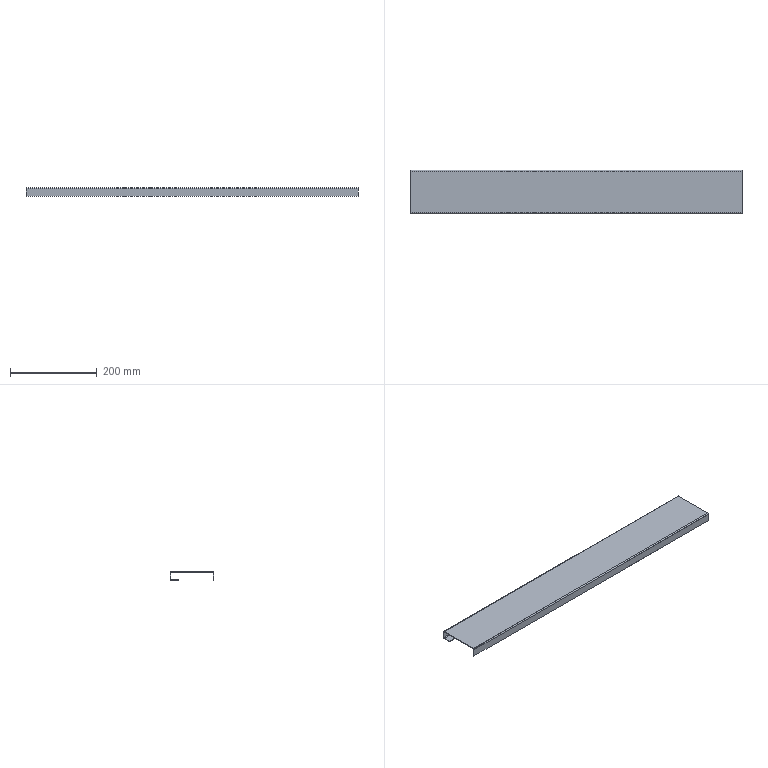Part | STEP file | E3-中转釜护栏7踢脚Plate | 1 solid | 18 faces | box 765 x 100 x 20 mm | volume 175851 mm3 | plane 12 | cylinder 6 | commonest cylinder face diameters 2 x3 5 x3
STEP:
#1=CARTESIAN_POINT('',(0.,0.,0.));
#2=DIRECTION('',(0.,0.,1.));
#3=DIRECTION('',(1.,0.,0.));
#4=AXIS2_PLACEMENT_3D('',#1,#2,#3);
#5=CARTESIAN_POINT('',(-382.5,1.5,-2.5));
#6=VERTEX_POINT('',#5);
#7=CARTESIAN_POINT('',(-382.5,1.5,-20.));
#8=VERTEX_POINT('',#7);
#9=CARTESIAN_POINT('',(-382.5,1.5,-2.5));
#10=DIRECTION('',(0.,0.,-1.));
#11=VECTOR('',#10,1.);
#12=LINE('',#9,#11);
#13=CARTESIAN_POINT('',(382.5,1.5,-2.5));
#14=DIRECTION('',(0.,-1.,0.));
#15=DIRECTION('',(0.,0.,1.));
#16=AXIS2_PLACEMENT_3D('',#13,#14,#15);
#17=PLANE('',#16);
#18=CARTESIAN_POINT('',(0.,765.));
#19=DIRECTION('',(-1.,0.));
#20=VECTOR('',#19,1.);
#21=LINE('',#18,#20);
#22=(GEOMETRIC_REPRESENTATION_CONTEXT(2)PARAMETRIC_REPRESENTATION_CONTEXT()REPRESENTATION_CONTEXT('',''));
#23=DEFINITIONAL_REPRESENTATION('',(#21),#22);
#24=PCURVE('',#17,#23);
#25=CARTESIAN_POINT('',(-382.5,2.5,-2.5));
#26=DIRECTION('',(-1.,0.,0.));
#27=DIRECTION('',(0.,0.,-1.));
#28=AXIS2_PLACEMENT_3D('',#25,#26,#27);
#29=PLANE('',#28);
#30=CARTESIAN_POINT('',(0.,1.));
#31=DIRECTION('',(1.,0.));
#32=VECTOR('',#31,1.);
#33=LINE('',#30,#32);
#34=(GEOMETRIC_REPRESENTATION_CONTEXT(2)PARAMETRIC_REPRESENTATION_CONTEXT()REPRESENTATION_CONTEXT('',''));
#35=DEFINITIONAL_REPRESENTATION('',(#33),#34);
#36=PCURVE('',#29,#35);
#37=SURFACE_CURVE('',#12,(#24,#36),.PCURVE_S1.);
#38=EDGE_CURVE('',#6,#8,#37,.T.);
#39=ORIENTED_EDGE('',*,*,#38,.F.);
#40=CARTESIAN_POINT('',(382.5,1.5,-2.5));
#41=VERTEX_POINT('',#40);
#42=CARTESIAN_POINT('',(382.5,1.5,-2.5));
#43=DIRECTION('',(-1.,0.,0.));
#44=VECTOR('',#43,1.);
#45=LINE('',#42,#44);
#46=CARTESIAN_POINT('',(0.,0.));
#47=DIRECTION('',(0.,1.));
#48=VECTOR('',#47,1.);
#49=LINE('',#46,#48);
#50=(GEOMETRIC_REPRESENTATION_CONTEXT(2)PARAMETRIC_REPRESENTATION_CONTEXT()REPRESENTATION_CONTEXT('',''));
#51=DEFINITIONAL_REPRESENTATION('',(#49),#50);
#52=PCURVE('',#17,#51);
#53=CARTESIAN_POINT('',(382.5,2.5,-2.5));
#54=DIRECTION('',(-1.,0.,0.));
#55=DIRECTION('',(0.,0.,-1.));
#56=AXIS2_PLACEMENT_3D('',#53,#54,#55);
#57=CYLINDRICAL_SURFACE('',#56,1.);
#58=CARTESIAN_POINT('',(1.571,0.));
#59=DIRECTION('',(0.,1.));
#60=VECTOR('',#59,1.);
#61=LINE('',#58,#60);
#62=(GEOMETRIC_REPRESENTATION_CONTEXT(2)PARAMETRIC_REPRESENTATION_CONTEXT()REPRESENTATION_CONTEXT('',''));
#63=DEFINITIONAL_REPRESENTATION('',(#61),#62);
#64=PCURVE('',#57,#63);
#65=SURFACE_CURVE('',#45,(#52,#64),.PCURVE_S1.);
#66=EDGE_CURVE('',#41,#6,#65,.T.);
#67=ORIENTED_EDGE('',*,*,#66,.F.);
#68=CARTESIAN_POINT('',(382.5,1.5,-20.));
#69=VERTEX_POINT('',#68);
#70=CARTESIAN_POINT('',(382.5,1.5,-2.5));
#71=DIRECTION('',(0.,0.,-1.));
#72=VECTOR('',#71,1.);
#73=LINE('',#70,#72);
#74=CARTESIAN_POINT('',(0.,0.));
#75=DIRECTION('',(-1.,0.));
#76=VECTOR('',#75,1.);
#77=LINE('',#74,#76);
#78=(GEOMETRIC_REPRESENTATION_CONTEXT(2)PARAMETRIC_REPRESENTATION_CONTEXT()REPRESENTATION_CONTEXT('',''));
#79=DEFINITIONAL_REPRESENTATION('',(#77),#78);
#80=PCURVE('',#17,#79);
#81=CARTESIAN_POINT('',(382.5,2.5,-2.5));
#82=DIRECTION('',(-1.,0.,0.));
#83=DIRECTION('',(0.,0.,-1.));
#84=AXIS2_PLACEMENT_3D('',#81,#82,#83);
#85=PLANE('',#84);
#86=CARTESIAN_POINT('',(0.,1.));
#87=DIRECTION('',(1.,0.));
#88=VECTOR('',#87,1.);
#89=LINE('',#86,#88);
#90=(GEOMETRIC_REPRESENTATION_CONTEXT(2)PARAMETRIC_REPRESENTATION_CONTEXT()REPRESENTATION_CONTEXT('',''));
#91=DEFINITIONAL_REPRESENTATION('',(#89),#90);
#92=PCURVE('',#85,#91);
#93=SURFACE_CURVE('',#73,(#80,#92),.PCURVE_S1.);
#94=EDGE_CURVE('',#41,#69,#93,.T.);
#95=ORIENTED_EDGE('',*,*,#94,.T.);
#96=CARTESIAN_POINT('',(382.5,1.5,-20.));
#97=DIRECTION('',(-1.,0.,0.));
#98=VECTOR('',#97,1.);
#99=LINE('',#96,#98);
#100=CARTESIAN_POINT('',(-17.5,0.));
#101=DIRECTION('',(0.,1.));
#102=VECTOR('',#101,1.);
#103=LINE('',#100,#102);
#104=(GEOMETRIC_REPRESENTATION_CONTEXT(2)PARAMETRIC_REPRESENTATION_CONTEXT()REPRESENTATION_CONTEXT('',''));
#105=DEFINITIONAL_REPRESENTATION('',(#103),#104);
#106=PCURVE('',#17,#105);
#107=CARTESIAN_POINT('',(382.5,0.,-20.));
#108=DIRECTION('',(0.,0.,-1.));
#109=DIRECTION('',(1.,0.,0.));
#110=AXIS2_PLACEMENT_3D('',#107,#108,#109);
#111=PLANE('',#110);
#112=CARTESIAN_POINT('',(0.,-1.5));
#113=DIRECTION('',(-1.,0.));
#114=VECTOR('',#113,1.);
#115=LINE('',#112,#114);
#116=(GEOMETRIC_REPRESENTATION_CONTEXT(2)PARAMETRIC_REPRESENTATION_CONTEXT()REPRESENTATION_CONTEXT('',''));
#117=DEFINITIONAL_REPRESENTATION('',(#115),#116);
#118=PCURVE('',#111,#117);
#119=SURFACE_CURVE('',#99,(#106,#118),.PCURVE_S1.);
#120=EDGE_CURVE('',#69,#8,#119,.T.);
#121=ORIENTED_EDGE('',*,*,#120,.T.);
#122=EDGE_LOOP('',(#39,#67,#95,#121));
#123=FACE_BOUND('',#122,.T.);
#124=ADVANCED_FACE('',(#123),#17,.F.);
#125=CARTESIAN_POINT('',(-382.5,0.,-20.));
#126=VERTEX_POINT('',#125);
#127=CARTESIAN_POINT('',(-382.5,0.,-20.));
#128=DIRECTION('',(0.,1.,0.));
#129=VECTOR('',#128,1.);
#130=LINE('',#127,#129);
#131=CARTESIAN_POINT('',(-765.,0.));
#132=DIRECTION('',(0.,-1.));
#133=VECTOR('',#132,1.);
#134=LINE('',#131,#133);
#135=(GEOMETRIC_REPRESENTATION_CONTEXT(2)PARAMETRIC_REPRESENTATION_CONTEXT()REPRESENTATION_CONTEXT('',''));
#136=DEFINITIONAL_REPRESENTATION('',(#134),#135);
#137=PCURVE('',#111,#136);
#138=CARTESIAN_POINT('',(17.5,2.5));
#139=DIRECTION('',(0.,-1.));
#140=VECTOR('',#139,1.);
#141=LINE('',#138,#140);
#142=(GEOMETRIC_REPRESENTATION_CONTEXT(2)PARAMETRIC_REPRESENTATION_CONTEXT()REPRESENTATION_CONTEXT('',''));
#143=DEFINITIONAL_REPRESENTATION('',(#141),#142);
#144=PCURVE('',#29,#143);
#145=SURFACE_CURVE('',#130,(#137,#144),.PCURVE_S1.);
#146=EDGE_CURVE('',#126,#8,#145,.T.);
#147=ORIENTED_EDGE('',*,*,#146,.T.);
#148=ORIENTED_EDGE('',*,*,#120,.F.);
#149=CARTESIAN_POINT('',(382.5,0.,-20.));
#150=VERTEX_POINT('',#149);
#151=CARTESIAN_POINT('',(382.5,0.,-20.));
#152=DIRECTION('',(0.,1.,0.));
#153=VECTOR('',#152,1.);
#154=LINE('',#151,#153);
#155=CARTESIAN_POINT('',(0.,0.));
#156=DIRECTION('',(0.,-1.));
#157=VECTOR('',#156,1.);
#158=LINE('',#155,#157);
#159=(GEOMETRIC_REPRESENTATION_CONTEXT(2)PARAMETRIC_REPRESENTATION_CONTEXT()REPRESENTATION_CONTEXT('',''));
#160=DEFINITIONAL_REPRESENTATION('',(#158),#159);
#161=PCURVE('',#111,#160);
#162=CARTESIAN_POINT('',(17.5,2.5));
#163=DIRECTION('',(0.,-1.));
#164=VECTOR('',#163,1.);
#165=LINE('',#162,#164);
#166=(GEOMETRIC_REPRESENTATION_CONTEXT(2)PARAMETRIC_REPRESENTATION_CONTEXT()REPRESENTATION_CONTEXT('',''));
#167=DEFINITIONAL_REPRESENTATION('',(#165),#166);
#168=PCURVE('',#85,#167);
#169=SURFACE_CURVE('',#154,(#161,#168),.PCURVE_S1.);
#170=EDGE_CURVE('',#150,#69,#169,.T.);
#171=ORIENTED_EDGE('',*,*,#170,.F.);
#172=CARTESIAN_POINT('',(382.5,0.,-20.));
#173=DIRECTION('',(-1.,0.,0.));
#174=VECTOR('',#173,1.);
#175=LINE('',#172,#174);
#176=CARTESIAN_POINT('',(0.,0.));
#177=DIRECTION('',(-1.,0.));
#178=VECTOR('',#177,1.);
#179=LINE('',#176,#178);
#180=(GEOMETRIC_REPRESENTATION_CONTEXT(2)PARAMETRIC_REPRESENTATION_CONTEXT()REPRESENTATION_CONTEXT('',''));
#181=DEFINITIONAL_REPRESENTATION('',(#179),#180);
#182=PCURVE('',#111,#181);
#183=CARTESIAN_POINT('',(382.5,0.,-2.5));
#184=DIRECTION('',(0.,-1.,0.));
#185=DIRECTION('',(0.,0.,1.));
#186=AXIS2_PLACEMENT_3D('',#183,#184,#185);
#187=PLANE('',#186);
#188=CARTESIAN_POINT('',(-17.5,0.));
#189=DIRECTION('',(0.,1.));
#190=VECTOR('',#189,1.);
#191=LINE('',#188,#190);
#192=(GEOMETRIC_REPRESENTATION_CONTEXT(2)PARAMETRIC_REPRESENTATION_CONTEXT()REPRESENTATION_CONTEXT('',''));
#193=DEFINITIONAL_REPRESENTATION('',(#191),#192);
#194=PCURVE('',#187,#193);
#195=SURFACE_CURVE('',#175,(#182,#194),.PCURVE_S1.);
#196=EDGE_CURVE('',#150,#126,#195,.T.);
#197=ORIENTED_EDGE('',*,*,#196,.T.);
#198=EDGE_LOOP('',(#147,#148,#171,#197));
#199=FACE_BOUND('',#198,.T.);
#200=ADVANCED_FACE('',(#199),#111,.T.);
#201=CARTESIAN_POINT('',(-382.5,0.,-2.5));
#202=VERTEX_POINT('',#201);
#203=CARTESIAN_POINT('',(-382.5,0.,-2.5));
#204=DIRECTION('',(0.,0.,-1.));
#205=VECTOR('',#204,1.);
#206=LINE('',#203,#205);
#207=CARTESIAN_POINT('',(0.,765.));
#208=DIRECTION('',(-1.,0.));
#209=VECTOR('',#208,1.);
#210=LINE('',#207,#209);
#211=(GEOMETRIC_REPRESENTATION_CONTEXT(2)PARAMETRIC_REPRESENTATION_CONTEXT()REPRESENTATION_CONTEXT('',''));
#212=DEFINITIONAL_REPRESENTATION('',(#210),#211);
#213=PCURVE('',#187,#212);
#214=CARTESIAN_POINT('',(0.,2.5));
#215=DIRECTION('',(1.,0.));
#216=VECTOR('',#215,1.);
#217=LINE('',#214,#216);
#218=(GEOMETRIC_REPRESENTATION_CONTEXT(2)PARAMETRIC_REPRESENTATION_CONTEXT()REPRESENTATION_CONTEXT('',''));
#219=DEFINITIONAL_REPRESENTATION('',(#217),#218);
#220=PCURVE('',#29,#219);
#221=SURFACE_CURVE('',#206,(#213,#220),.PCURVE_S1.);
#222=EDGE_CURVE('',#202,#126,#221,.T.);
#223=ORIENTED_EDGE('',*,*,#222,.T.);
#224=ORIENTED_EDGE('',*,*,#196,.F.);
#225=CARTESIAN_POINT('',(382.5,0.,-2.5));
#226=VERTEX_POINT('',#225);
#227=CARTESIAN_POINT('',(382.5,0.,-2.5));
#228=DIRECTION('',(0.,0.,-1.));
#229=VECTOR('',#228,1.);
#230=LINE('',#227,#229);
#231=CARTESIAN_POINT('',(0.,0.));
#232=DIRECTION('',(-1.,0.));
#233=VECTOR('',#232,1.);
#234=LINE('',#231,#233);
#235=(GEOMETRIC_REPRESENTATION_CONTEXT(2)PARAMETRIC_REPRESENTATION_CONTEXT()REPRESENTATION_CONTEXT('',''));
#236=DEFINITIONAL_REPRESENTATION('',(#234),#235);
#237=PCURVE('',#187,#236);
#238=CARTESIAN_POINT('',(0.,2.5));
#239=DIRECTION('',(1.,0.));
#240=VECTOR('',#239,1.);
#241=LINE('',#238,#240);
#242=(GEOMETRIC_REPRESENTATION_CONTEXT(2)PARAMETRIC_REPRESENTATION_CONTEXT()REPRESENTATION_CONTEXT('',''));
#243=DEFINITIONAL_REPRESENTATION('',(#241),#242);
#244=PCURVE('',#85,#243);
#245=SURFACE_CURVE('',#230,(#237,#244),.PCURVE_S1.);
#246=EDGE_CURVE('',#226,#150,#245,.T.);
#247=ORIENTED_EDGE('',*,*,#246,.F.);
#248=CARTESIAN_POINT('',(382.5,0.,-2.5));
#249=DIRECTION('',(-1.,0.,0.));
#250=VECTOR('',#249,1.);
#251=LINE('',#248,#250);
#252=CARTESIAN_POINT('',(0.,0.));
#253=DIRECTION('',(0.,1.));
#254=VECTOR('',#253,1.);
#255=LINE('',#252,#254);
#256=(GEOMETRIC_REPRESENTATION_CONTEXT(2)PARAMETRIC_REPRESENTATION_CONTEXT()REPRESENTATION_CONTEXT('',''));
#257=DEFINITIONAL_REPRESENTATION('',(#255),#256);
#258=PCURVE('',#187,#257);
#259=CARTESIAN_POINT('',(382.5,2.5,-2.5));
#260=DIRECTION('',(-1.,0.,0.));
#261=DIRECTION('',(0.,0.,-1.));
#262=AXIS2_PLACEMENT_3D('',#259,#260,#261);
#263=CYLINDRICAL_SURFACE('',#262,2.5);
#264=CARTESIAN_POINT('',(1.571,0.));
#265=DIRECTION('',(0.,1.));
#266=VECTOR('',#265,1.);
#267=LINE('',#264,#266);
#268=(GEOMETRIC_REPRESENTATION_CONTEXT(2)PARAMETRIC_REPRESENTATION_CONTEXT()REPRESENTATION_CONTEXT('',''));
#269=DEFINITIONAL_REPRESENTATION('',(#267),#268);
#270=PCURVE('',#263,#269);
#271=SURFACE_CURVE('',#251,(#258,#270),.PCURVE_S1.);
#272=EDGE_CURVE('',#226,#202,#271,.T.);
#273=ORIENTED_EDGE('',*,*,#272,.T.);
#274=EDGE_LOOP('',(#223,#224,#247,#273));
#275=FACE_BOUND('',#274,.T.);
#276=ADVANCED_FACE('',(#275),#187,.T.);
#277=CARTESIAN_POINT('',(-382.5,2.5,0.));
#278=VERTEX_POINT('',#277);
#279=CARTESIAN_POINT('',(-382.5,2.5,-2.5));
#280=DIRECTION('',(1.,0.,0.));
#281=DIRECTION('',(0.,0.,-1.));
#282=AXIS2_PLACEMENT_3D('',#279,#280,#281);
#283=CIRCLE('',#282,2.5);
#284=CARTESIAN_POINT('',(6.283,765.));
#285=DIRECTION('',(-1.,0.));
#286=VECTOR('',#285,1.);
#287=LINE('',#284,#286);
#288=(GEOMETRIC_REPRESENTATION_CONTEXT(2)PARAMETRIC_REPRESENTATION_CONTEXT()REPRESENTATION_CONTEXT('',''));
#289=DEFINITIONAL_REPRESENTATION('',(#287),#288);
#290=PCURVE('',#263,#289);
#291=CARTESIAN_POINT('',(2.5,0.));
#292=CARTESIAN_POINT('',(2.5,-4.33));
#293=CARTESIAN_POINT('',(-1.25,-2.165));
#294=CARTESIAN_POINT('',(-5.,0.));
#295=CARTESIAN_POINT('',(-1.25,2.165));
#296=CARTESIAN_POINT('',(2.5,4.33));
#297=CARTESIAN_POINT('',(2.5,0.));
#298=(BOUNDED_CURVE()B_SPLINE_CURVE(2,(#291,#292,#293,#294,#295,#296,#297),.UNSPECIFIED.,.T.,.F.)B_SPLINE_CURVE_WITH_KNOTS((1,2,2,2,2,1),(-2.094,0.,2.094,4.189,6.283,8.378),.UNSPECIFIED.)CURVE()GEOMETRIC_REPRESENTATION_ITEM()RATIONAL_B_SPLINE_CURVE((1.,0.5,1.,0.5,1.,0.5,1.))REPRESENTATION_ITEM(''));
#299=(GEOMETRIC_REPRESENTATION_CONTEXT(2)PARAMETRIC_REPRESENTATION_CONTEXT()REPRESENTATION_CONTEXT('',''));
#300=DEFINITIONAL_REPRESENTATION('',(#298),#299);
#301=PCURVE('',#29,#300);
#302=SURFACE_CURVE('',#283,(#290,#301),.PCURVE_S1.);
#303=EDGE_CURVE('',#278,#202,#302,.T.);
#304=ORIENTED_EDGE('',*,*,#303,.T.);
#305=ORIENTED_EDGE('',*,*,#272,.F.);
#306=CARTESIAN_POINT('',(382.5,2.5,0.));
#307=VERTEX_POINT('',#306);
#308=CARTESIAN_POINT('',(382.5,2.5,-2.5));
#309=DIRECTION('',(1.,0.,0.));
#310=DIRECTION('',(0.,0.,-1.));
#311=AXIS2_PLACEMENT_3D('',#308,#309,#310);
#312=CIRCLE('',#311,2.5);
#313=CARTESIAN_POINT('',(6.283,0.));
#314=DIRECTION('',(-1.,0.));
#315=VECTOR('',#314,1.);
#316=LINE('',#313,#315);
#317=(GEOMETRIC_REPRESENTATION_CONTEXT(2)PARAMETRIC_REPRESENTATION_CONTEXT()REPRESENTATION_CONTEXT('',''));
#318=DEFINITIONAL_REPRESENTATION('',(#316),#317);
#319=PCURVE('',#263,#318);
#320=CARTESIAN_POINT('',(2.5,0.));
#321=CARTESIAN_POINT('',(2.5,-4.33));
#322=CARTESIAN_POINT('',(-1.25,-2.165));
#323=CARTESIAN_POINT('',(-5.,0.));
#324=CARTESIAN_POINT('',(-1.25,2.165));
#325=CARTESIAN_POINT('',(2.5,4.33));
#326=CARTESIAN_POINT('',(2.5,0.));
#327=(BOUNDED_CURVE()B_SPLINE_CURVE(2,(#320,#321,#322,#323,#324,#325,#326),.UNSPECIFIED.,.T.,.F.)B_SPLINE_CURVE_WITH_KNOTS((1,2,2,2,2,1),(-2.094,0.,2.094,4.189,6.283,8.378),.UNSPECIFIED.)CURVE()GEOMETRIC_REPRESENTATION_ITEM()RATIONAL_B_SPLINE_CURVE((1.,0.5,1.,0.5,1.,0.5,1.))REPRESENTATION_ITEM(''));
#328=(GEOMETRIC_REPRESENTATION_CONTEXT(2)PARAMETRIC_REPRESENTATION_CONTEXT()REPRESENTATION_CONTEXT('',''));
#329=DEFINITIONAL_REPRESENTATION('',(#327),#328);
#330=PCURVE('',#85,#329);
#331=SURFACE_CURVE('',#312,(#319,#330),.PCURVE_S1.);
#332=EDGE_CURVE('',#307,#226,#331,.T.);
#333=ORIENTED_EDGE('',*,*,#332,.F.);
#334=CARTESIAN_POINT('',(382.5,2.5,0.));
#335=DIRECTION('',(-1.,0.,0.));
#336=VECTOR('',#335,1.);
#337=LINE('',#334,#336);
#338=CARTESIAN_POINT('',(3.142,0.));
#339=DIRECTION('',(0.,1.));
#340=VECTOR('',#339,1.);
#341=LINE('',#338,#340);
#342=(GEOMETRIC_REPRESENTATION_CONTEXT(2)PARAMETRIC_REPRESENTATION_CONTEXT()REPRESENTATION_CONTEXT('',''));
#343=DEFINITIONAL_REPRESENTATION('',(#341),#342);
#344=PCURVE('',#263,#343);
#345=CARTESIAN_POINT('',(382.5,2.5,0.));
#346=DIRECTION('',(0.,0.,1.));
#347=DIRECTION('',(-1.,0.,0.));
#348=AXIS2_PLACEMENT_3D('',#345,#346,#347);
#349=PLANE('',#348);
#350=CARTESIAN_POINT('',(0.,0.));
#351=DIRECTION('',(1.,0.));
#352=VECTOR('',#351,1.);
#353=LINE('',#350,#352);
#354=(GEOMETRIC_REPRESENTATION_CONTEXT(2)PARAMETRIC_REPRESENTATION_CONTEXT()REPRESENTATION_CONTEXT('',''));
#355=DEFINITIONAL_REPRESENTATION('',(#353),#354);
#356=PCURVE('',#349,#355);
#357=SURFACE_CURVE('',#337,(#344,#356),.PCURVE_S1.);
#358=EDGE_CURVE('',#307,#278,#357,.T.);
#359=ORIENTED_EDGE('',*,*,#358,.T.);
#360=EDGE_LOOP('',(#304,#305,#333,#359));
#361=FACE_BOUND('',#360,.T.);
#362=ADVANCED_FACE('',(#361),#263,.T.);
#363=CARTESIAN_POINT('',(-382.5,97.5,0.));
#364=VERTEX_POINT('',#363);
#365=CARTESIAN_POINT('',(-382.5,2.5,0.));
#366=DIRECTION('',(0.,-1.,0.));
#367=VECTOR('',#366,1.);
#368=LINE('',#365,#367);
#369=CARTESIAN_POINT('',(765.,0.));
#370=DIRECTION('',(0.,1.));
#371=VECTOR('',#370,1.);
#372=LINE('',#369,#371);
#373=(GEOMETRIC_REPRESENTATION_CONTEXT(2)PARAMETRIC_REPRESENTATION_CONTEXT()REPRESENTATION_CONTEXT('',''));
#374=DEFINITIONAL_REPRESENTATION('',(#372),#373);
#375=PCURVE('',#349,#374);
#376=CARTESIAN_POINT('',(-2.5,0.));
#377=DIRECTION('',(0.,1.));
#378=VECTOR('',#377,1.);
#379=LINE('',#376,#378);
#380=(GEOMETRIC_REPRESENTATION_CONTEXT(2)PARAMETRIC_REPRESENTATION_CONTEXT()REPRESENTATION_CONTEXT('',''));
#381=DEFINITIONAL_REPRESENTATION('',(#379),#380);
#382=PCURVE('',#29,#381);
#383=SURFACE_CURVE('',#368,(#375,#382),.PCURVE_S1.);
#384=EDGE_CURVE('',#364,#278,#383,.T.);
#385=ORIENTED_EDGE('',*,*,#384,.T.);
#386=ORIENTED_EDGE('',*,*,#358,.F.);
#387=CARTESIAN_POINT('',(382.5,97.5,0.));
#388=VERTEX_POINT('',#387);
#389=CARTESIAN_POINT('',(382.5,2.5,0.));
#390=DIRECTION('',(0.,-1.,0.));
#391=VECTOR('',#390,1.);
#392=LINE('',#389,#391);
#393=CARTESIAN_POINT('',(0.,0.));
#394=DIRECTION('',(0.,1.));
#395=VECTOR('',#394,1.);
#396=LINE('',#393,#395);
#397=(GEOMETRIC_REPRESENTATION_CONTEXT(2)PARAMETRIC_REPRESENTATION_CONTEXT()REPRESENTATION_CONTEXT('',''));
#398=DEFINITIONAL_REPRESENTATION('',(#396),#397);
#399=PCURVE('',#349,#398);
#400=CARTESIAN_POINT('',(-2.5,0.));
#401=DIRECTION('',(0.,1.));
#402=VECTOR('',#401,1.);
#403=LINE('',#400,#402);
#404=(GEOMETRIC_REPRESENTATION_CONTEXT(2)PARAMETRIC_REPRESENTATION_CONTEXT()REPRESENTATION_CONTEXT('',''));
#405=DEFINITIONAL_REPRESENTATION('',(#403),#404);
#406=PCURVE('',#85,#405);
#407=SURFACE_CURVE('',#392,(#399,#406),.PCURVE_S1.);
#408=EDGE_CURVE('',#388,#307,#407,.T.);
#409=ORIENTED_EDGE('',*,*,#408,.F.);
#410=CARTESIAN_POINT('',(382.5,97.5,0.));
#411=DIRECTION('',(-1.,0.,0.));
#412=VECTOR('',#411,1.);
#413=LINE('',#410,#412);
#414=CARTESIAN_POINT('',(0.,-95.));
#415=DIRECTION('',(1.,0.));
#416=VECTOR('',#415,1.);
#417=LINE('',#414,#416);
#418=(GEOMETRIC_REPRESENTATION_CONTEXT(2)PARAMETRIC_REPRESENTATION_CONTEXT()REPRESENTATION_CONTEXT('',''));
#419=DEFINITIONAL_REPRESENTATION('',(#417),#418);
#420=PCURVE('',#349,#419);
#421=CARTESIAN_POINT('',(382.5,97.5,-2.5));
#422=DIRECTION('',(-1.,0.,0.));
#423=DIRECTION('',(0.,0.,-1.));
#424=AXIS2_PLACEMENT_3D('',#421,#422,#423);
#425=CYLINDRICAL_SURFACE('',#424,2.5);
#426=CARTESIAN_POINT('',(3.142,0.));
#427=DIRECTION('',(0.,1.));
#428=VECTOR('',#427,1.);
#429=LINE('',#426,#428);
#430=(GEOMETRIC_REPRESENTATION_CONTEXT(2)PARAMETRIC_REPRESENTATION_CONTEXT()REPRESENTATION_CONTEXT('',''));
#431=DEFINITIONAL_REPRESENTATION('',(#429),#430);
#432=PCURVE('',#425,#431);
#433=SURFACE_CURVE('',#413,(#420,#432),.PCURVE_S1.);
#434=EDGE_CURVE('',#388,#364,#433,.T.);
#435=ORIENTED_EDGE('',*,*,#434,.T.);
#436=EDGE_LOOP('',(#385,#386,#409,#435));
#437=FACE_BOUND('',#436,.T.);
#438=ADVANCED_FACE('',(#437),#349,.T.);
#439=CARTESIAN_POINT('',(-382.5,100.,-2.5));
#440=VERTEX_POINT('',#439);
#441=CARTESIAN_POINT('',(-382.5,97.5,-2.5));
#442=DIRECTION('',(1.,0.,0.));
#443=DIRECTION('',(0.,0.,1.));
#444=AXIS2_PLACEMENT_3D('',#441,#442,#443);
#445=CIRCLE('',#444,2.5);
#446=CARTESIAN_POINT('',(9.425,765.));
#447=DIRECTION('',(-1.,0.));
#448=VECTOR('',#447,1.);
#449=LINE('',#446,#448);
#450=(GEOMETRIC_REPRESENTATION_CONTEXT(2)PARAMETRIC_REPRESENTATION_CONTEXT()REPRESENTATION_CONTEXT('',''));
#451=DEFINITIONAL_REPRESENTATION('',(#449),#450);
#452=PCURVE('',#425,#451);
#453=CARTESIAN_POINT('',(-2.5,-95.));
#454=CARTESIAN_POINT('',(-2.5,-90.67));
#455=CARTESIAN_POINT('',(1.25,-92.835));
#456=CARTESIAN_POINT('',(5.,-95.));
#457=CARTESIAN_POINT('',(1.25,-97.165));
#458=CARTESIAN_POINT('',(-2.5,-99.33));
#459=CARTESIAN_POINT('',(-2.5,-95.));
#460=(BOUNDED_CURVE()B_SPLINE_CURVE(2,(#453,#454,#455,#456,#457,#458,#459),.UNSPECIFIED.,.T.,.F.)B_SPLINE_CURVE_WITH_KNOTS((1,2,2,2,2,1),(-2.094,0.,2.094,4.189,6.283,8.378),.UNSPECIFIED.)CURVE()GEOMETRIC_REPRESENTATION_ITEM()RATIONAL_B_SPLINE_CURVE((1.,0.5,1.,0.5,1.,0.5,1.))REPRESENTATION_ITEM(''));
#461=(GEOMETRIC_REPRESENTATION_CONTEXT(2)PARAMETRIC_REPRESENTATION_CONTEXT()REPRESENTATION_CONTEXT('',''));
#462=DEFINITIONAL_REPRESENTATION('',(#460),#461);
#463=PCURVE('',#29,#462);
#464=SURFACE_CURVE('',#445,(#452,#463),.PCURVE_S1.);
#465=EDGE_CURVE('',#440,#364,#464,.T.);
#466=ORIENTED_EDGE('',*,*,#465,.T.);
#467=ORIENTED_EDGE('',*,*,#434,.F.);
#468=CARTESIAN_POINT('',(382.5,100.,-2.5));
#469=VERTEX_POINT('',#468);
#470=CARTESIAN_POINT('',(382.5,97.5,-2.5));
#471=DIRECTION('',(1.,0.,0.));
#472=DIRECTION('',(0.,0.,1.));
#473=AXIS2_PLACEMENT_3D('',#470,#471,#472);
#474=CIRCLE('',#473,2.5);
#475=CARTESIAN_POINT('',(9.425,0.));
#476=DIRECTION('',(-1.,0.));
#477=VECTOR('',#476,1.);
#478=LINE('',#475,#477);
#479=(GEOMETRIC_REPRESENTATION_CONTEXT(2)PARAMETRIC_REPRESENTATION_CONTEXT()REPRESENTATION_CONTEXT('',''));
#480=DEFINITIONAL_REPRESENTATION('',(#478),#479);
#481=PCURVE('',#425,#480);
#482=CARTESIAN_POINT('',(-2.5,-95.));
#483=CARTESIAN_POINT('',(-2.5,-90.67));
#484=CARTESIAN_POINT('',(1.25,-92.835));
#485=CARTESIAN_POINT('',(5.,-95.));
#486=CARTESIAN_POINT('',(1.25,-97.165));
#487=CARTESIAN_POINT('',(-2.5,-99.33));
#488=CARTESIAN_POINT('',(-2.5,-95.));
#489=(BOUNDED_CURVE()B_SPLINE_CURVE(2,(#482,#483,#484,#485,#486,#487,#488),.UNSPECIFIED.,.T.,.F.)B_SPLINE_CURVE_WITH_KNOTS((1,2,2,2,2,1),(-2.094,0.,2.094,4.189,6.283,8.378),.UNSPECIFIED.)CURVE()GEOMETRIC_REPRESENTATION_ITEM()RATIONAL_B_SPLINE_CURVE((1.,0.5,1.,0.5,1.,0.5,1.))REPRESENTATION_ITEM(''));
#490=(GEOMETRIC_REPRESENTATION_CONTEXT(2)PARAMETRIC_REPRESENTATION_CONTEXT()REPRESENTATION_CONTEXT('',''));
#491=DEFINITIONAL_REPRESENTATION('',(#489),#490);
#492=PCURVE('',#85,#491);
#493=SURFACE_CURVE('',#474,(#481,#492),.PCURVE_S1.);
#494=EDGE_CURVE('',#469,#388,#493,.T.);
#495=ORIENTED_EDGE('',*,*,#494,.F.);
#496=CARTESIAN_POINT('',(382.5,100.,-2.5));
#497=DIRECTION('',(-1.,0.,0.));
#498=VECTOR('',#497,1.);
#499=LINE('',#496,#498);
#500=CARTESIAN_POINT('',(4.712,0.));
#501=DIRECTION('',(0.,1.));
#502=VECTOR('',#501,1.);
#503=LINE('',#500,#502);
#504=(GEOMETRIC_REPRESENTATION_CONTEXT(2)PARAMETRIC_REPRESENTATION_CONTEXT()REPRESENTATION_CONTEXT('',''));
#505=DEFINITIONAL_REPRESENTATION('',(#503),#504);
#506=PCURVE('',#425,#505);
#507=CARTESIAN_POINT('',(382.5,100.,-2.5));
#508=DIRECTION('',(0.,1.,0.));
#509=DIRECTION('',(0.,0.,-1.));
#510=AXIS2_PLACEMENT_3D('',#507,#508,#509);
#511=PLANE('',#510);
#512=CARTESIAN_POINT('',(0.,0.));
#513=DIRECTION('',(0.,1.));
#514=VECTOR('',#513,1.);
#515=LINE('',#512,#514);
#516=(GEOMETRIC_REPRESENTATION_CONTEXT(2)PARAMETRIC_REPRESENTATION_CONTEXT()REPRESENTATION_CONTEXT('',''));
#517=DEFINITIONAL_REPRESENTATION('',(#515),#516);
#518=PCURVE('',#511,#517);
#519=SURFACE_CURVE('',#499,(#506,#518),.PCURVE_S1.);
#520=EDGE_CURVE('',#469,#440,#519,.T.);
#521=ORIENTED_EDGE('',*,*,#520,.T.);
#522=EDGE_LOOP('',(#466,#467,#495,#521));
#523=FACE_BOUND('',#522,.T.);
#524=ADVANCED_FACE('',(#523),#425,.T.);
#525=CARTESIAN_POINT('',(-382.5,100.,-17.5));
#526=VERTEX_POINT('',#525);
#527=CARTESIAN_POINT('',(-382.5,100.,-2.5));
#528=DIRECTION('',(0.,0.,1.));
#529=VECTOR('',#528,1.);
#530=LINE('',#527,#529);
#531=CARTESIAN_POINT('',(0.,765.));
#532=DIRECTION('',(-1.,0.));
#533=VECTOR('',#532,1.);
#534=LINE('',#531,#533);
#535=(GEOMETRIC_REPRESENTATION_CONTEXT(2)PARAMETRIC_REPRESENTATION_CONTEXT()REPRESENTATION_CONTEXT('',''));
#536=DEFINITIONAL_REPRESENTATION('',(#534),#535);
#537=PCURVE('',#511,#536);
#538=CARTESIAN_POINT('',(0.,-97.5));
#539=DIRECTION('',(-1.,0.));
#540=VECTOR('',#539,1.);
#541=LINE('',#538,#540);
#542=(GEOMETRIC_REPRESENTATION_CONTEXT(2)PARAMETRIC_REPRESENTATION_CONTEXT()REPRESENTATION_CONTEXT('',''));
#543=DEFINITIONAL_REPRESENTATION('',(#541),#542);
#544=PCURVE('',#29,#543);
#545=SURFACE_CURVE('',#530,(#537,#544),.PCURVE_S1.);
#546=EDGE_CURVE('',#526,#440,#545,.T.);
#547=ORIENTED_EDGE('',*,*,#546,.T.);
#548=ORIENTED_EDGE('',*,*,#520,.F.);
#549=CARTESIAN_POINT('',(382.5,100.,-17.5));
#550=VERTEX_POINT('',#549);
#551=CARTESIAN_POINT('',(382.5,100.,-2.5));
#552=DIRECTION('',(0.,0.,1.));
#553=VECTOR('',#552,1.);
#554=LINE('',#551,#553);
#555=CARTESIAN_POINT('',(0.,0.));
#556=DIRECTION('',(-1.,0.));
#557=VECTOR('',#556,1.);
#558=LINE('',#555,#557);
#559=(GEOMETRIC_REPRESENTATION_CONTEXT(2)PARAMETRIC_REPRESENTATION_CONTEXT()REPRESENTATION_CONTEXT('',''));
#560=DEFINITIONAL_REPRESENTATION('',(#558),#559);
#561=PCURVE('',#511,#560);
#562=CARTESIAN_POINT('',(0.,-97.5));
#563=DIRECTION('',(-1.,0.));
#564=VECTOR('',#563,1.);
#565=LINE('',#562,#564);
#566=(GEOMETRIC_REPRESENTATION_CONTEXT(2)PARAMETRIC_REPRESENTATION_CONTEXT()REPRESENTATION_CONTEXT('',''));
#567=DEFINITIONAL_REPRESENTATION('',(#565),#566);
#568=PCURVE('',#85,#567);
#569=SURFACE_CURVE('',#554,(#561,#568),.PCURVE_S1.);
#570=EDGE_CURVE('',#550,#469,#569,.T.);
#571=ORIENTED_EDGE('',*,*,#570,.F.);
#572=CARTESIAN_POINT('',(382.5,100.,-17.5));
#573=DIRECTION('',(-1.,0.,0.));
#574=VECTOR('',#573,1.);
#575=LINE('',#572,#574);
#576=CARTESIAN_POINT('',(15.,0.));
#577=DIRECTION('',(0.,1.));
#578=VECTOR('',#577,1.);
#579=LINE('',#576,#578);
#580=(GEOMETRIC_REPRESENTATION_CONTEXT(2)PARAMETRIC_REPRESENTATION_CONTEXT()REPRESENTATION_CONTEXT('',''));
#581=DEFINITIONAL_REPRESENTATION('',(#579),#580);
#582=PCURVE('',#511,#581);
#583=CARTESIAN_POINT('',(382.5,97.5,-17.5));
#584=DIRECTION('',(-1.,0.,0.));
#585=DIRECTION('',(0.,0.,-1.));
#586=AXIS2_PLACEMENT_3D('',#583,#584,#585);
#587=CYLINDRICAL_SURFACE('',#586,2.5);
#588=CARTESIAN_POINT('',(4.712,0.));
#589=DIRECTION('',(0.,1.));
#590=VECTOR('',#589,1.);
#591=LINE('',#588,#590);
#592=(GEOMETRIC_REPRESENTATION_CONTEXT(2)PARAMETRIC_REPRESENTATION_CONTEXT()REPRESENTATION_CONTEXT('',''));
#593=DEFINITIONAL_REPRESENTATION('',(#591),#592);
#594=PCURVE('',#587,#593);
#595=SURFACE_CURVE('',#575,(#582,#594),.PCURVE_S1.);
#596=EDGE_CURVE('',#550,#526,#595,.T.);
#597=ORIENTED_EDGE('',*,*,#596,.T.);
#598=EDGE_LOOP('',(#547,#548,#571,#597));
#599=FACE_BOUND('',#598,.T.);
#600=ADVANCED_FACE('',(#599),#511,.T.);
#601=CARTESIAN_POINT('',(-382.5,97.5,-20.));
#602=VERTEX_POINT('',#601);
#603=CARTESIAN_POINT('',(-382.5,97.5,-17.5));
#604=DIRECTION('',(1.,0.,0.));
#605=DIRECTION('',(0.,0.,1.));
#606=AXIS2_PLACEMENT_3D('',#603,#604,#605);
#607=CIRCLE('',#606,2.5);
#608=CARTESIAN_POINT('',(9.425,765.));
#609=DIRECTION('',(-1.,0.));
#610=VECTOR('',#609,1.);
#611=LINE('',#608,#610);
#612=(GEOMETRIC_REPRESENTATION_CONTEXT(2)PARAMETRIC_REPRESENTATION_CONTEXT()REPRESENTATION_CONTEXT('',''));
#613=DEFINITIONAL_REPRESENTATION('',(#611),#612);
#614=PCURVE('',#587,#613);
#615=CARTESIAN_POINT('',(12.5,-95.));
#616=CARTESIAN_POINT('',(12.5,-90.67));
#617=CARTESIAN_POINT('',(16.25,-92.835));
#618=CARTESIAN_POINT('',(20.,-95.));
#619=CARTESIAN_POINT('',(16.25,-97.165));
#620=CARTESIAN_POINT('',(12.5,-99.33));
#621=CARTESIAN_POINT('',(12.5,-95.));
#622=(BOUNDED_CURVE()B_SPLINE_CURVE(2,(#615,#616,#617,#618,#619,#620,#621),.UNSPECIFIED.,.T.,.F.)B_SPLINE_CURVE_WITH_KNOTS((1,2,2,2,2,1),(-2.094,0.,2.094,4.189,6.283,8.378),.UNSPECIFIED.)CURVE()GEOMETRIC_REPRESENTATION_ITEM()RATIONAL_B_SPLINE_CURVE((1.,0.5,1.,0.5,1.,0.5,1.))REPRESENTATION_ITEM(''));
#623=(GEOMETRIC_REPRESENTATION_CONTEXT(2)PARAMETRIC_REPRESENTATION_CONTEXT()REPRESENTATION_CONTEXT('',''));
#624=DEFINITIONAL_REPRESENTATION('',(#622),#623);
#625=PCURVE('',#29,#624);
#626=SURFACE_CURVE('',#607,(#614,#625),.PCURVE_S1.);
#627=EDGE_CURVE('',#602,#526,#626,.T.);
#628=ORIENTED_EDGE('',*,*,#627,.T.);
#629=ORIENTED_EDGE('',*,*,#596,.F.);
#630=CARTESIAN_POINT('',(382.5,97.5,-20.));
#631=VERTEX_POINT('',#630);
#632=CARTESIAN_POINT('',(382.5,97.5,-17.5));
#633=DIRECTION('',(1.,0.,0.));
#634=DIRECTION('',(0.,0.,1.));
#635=AXIS2_PLACEMENT_3D('',#632,#633,#634);
#636=CIRCLE('',#635,2.5);
#637=CARTESIAN_POINT('',(9.425,0.));
#638=DIRECTION('',(-1.,0.));
#639=VECTOR('',#638,1.);
#640=LINE('',#637,#639);
#641=(GEOMETRIC_REPRESENTATION_CONTEXT(2)PARAMETRIC_REPRESENTATION_CONTEXT()REPRESENTATION_CONTEXT('',''));
#642=DEFINITIONAL_REPRESENTATION('',(#640),#641);
#643=PCURVE('',#587,#642);
#644=CARTESIAN_POINT('',(12.5,-95.));
#645=CARTESIAN_POINT('',(12.5,-90.67));
#646=CARTESIAN_POINT('',(16.25,-92.835));
#647=CARTESIAN_POINT('',(20.,-95.));
#648=CARTESIAN_POINT('',(16.25,-97.165));
#649=CARTESIAN_POINT('',(12.5,-99.33));
#650=CARTESIAN_POINT('',(12.5,-95.));
#651=(BOUNDED_CURVE()B_SPLINE_CURVE(2,(#644,#645,#646,#647,#648,#649,#650),.UNSPECIFIED.,.T.,.F.)B_SPLINE_CURVE_WITH_KNOTS((1,2,2,2,2,1),(-2.094,0.,2.094,4.189,6.283,8.378),.UNSPECIFIED.)CURVE()GEOMETRIC_REPRESENTATION_ITEM()RATIONAL_B_SPLINE_CURVE((1.,0.5,1.,0.5,1.,0.5,1.))REPRESENTATION_ITEM(''));
#652=(GEOMETRIC_REPRESENTATION_CONTEXT(2)PARAMETRIC_REPRESENTATION_CONTEXT()REPRESENTATION_CONTEXT('',''));
#653=DEFINITIONAL_REPRESENTATION('',(#651),#652);
#654=PCURVE('',#85,#653);
#655=SURFACE_CURVE('',#636,(#643,#654),.PCURVE_S1.);
#656=EDGE_CURVE('',#631,#550,#655,.T.);
#657=ORIENTED_EDGE('',*,*,#656,.F.);
#658=CARTESIAN_POINT('',(382.5,97.5,-20.));
#659=DIRECTION('',(-1.,0.,0.));
#660=VECTOR('',#659,1.);
#661=LINE('',#658,#660);
#662=CARTESIAN_POINT('',(6.283,0.));
#663=DIRECTION('',(0.,1.));
#664=VECTOR('',#663,1.);
#665=LINE('',#662,#664);
#666=(GEOMETRIC_REPRESENTATION_CONTEXT(2)PARAMETRIC_REPRESENTATION_CONTEXT()REPRESENTATION_CONTEXT('',''));
#667=DEFINITIONAL_REPRESENTATION('',(#665),#666);
#668=PCURVE('',#587,#667);
#669=CARTESIAN_POINT('',(382.5,97.5,-20.));
#670=DIRECTION('',(0.,0.,-1.));
#671=DIRECTION('',(1.,0.,0.));
#672=AXIS2_PLACEMENT_3D('',#669,#670,#671);
#673=PLANE('',#672);
#674=CARTESIAN_POINT('',(0.,0.));
#675=DIRECTION('',(-1.,0.));
#676=VECTOR('',#675,1.);
#677=LINE('',#674,#676);
#678=(GEOMETRIC_REPRESENTATION_CONTEXT(2)PARAMETRIC_REPRESENTATION_CONTEXT()REPRESENTATION_CONTEXT('',''));
#679=DEFINITIONAL_REPRESENTATION('',(#677),#678);
#680=PCURVE('',#673,#679);
#681=SURFACE_CURVE('',#661,(#668,#680),.PCURVE_S1.);
#682=EDGE_CURVE('',#631,#602,#681,.T.);
#683=ORIENTED_EDGE('',*,*,#682,.T.);
#684=EDGE_LOOP('',(#628,#629,#657,#683));
#685=FACE_BOUND('',#684,.T.);
#686=ADVANCED_FACE('',(#685),#587,.T.);
#687=CARTESIAN_POINT('',(-382.5,80.,-20.));
#688=VERTEX_POINT('',#687);
#689=CARTESIAN_POINT('',(-382.5,97.5,-20.));
#690=DIRECTION('',(0.,1.,0.));
#691=VECTOR('',#690,1.);
#692=LINE('',#689,#691);
#693=CARTESIAN_POINT('',(-765.,0.));
#694=DIRECTION('',(0.,-1.));
#695=VECTOR('',#694,1.);
#696=LINE('',#693,#695);
#697=(GEOMETRIC_REPRESENTATION_CONTEXT(2)PARAMETRIC_REPRESENTATION_CONTEXT()REPRESENTATION_CONTEXT('',''));
#698=DEFINITIONAL_REPRESENTATION('',(#696),#697);
#699=PCURVE('',#673,#698);
#700=CARTESIAN_POINT('',(17.5,-95.));
#701=DIRECTION('',(0.,-1.));
#702=VECTOR('',#701,1.);
#703=LINE('',#700,#702);
#704=(GEOMETRIC_REPRESENTATION_CONTEXT(2)PARAMETRIC_REPRESENTATION_CONTEXT()REPRESENTATION_CONTEXT('',''));
#705=DEFINITIONAL_REPRESENTATION('',(#703),#704);
#706=PCURVE('',#29,#705);
#707=SURFACE_CURVE('',#692,(#699,#706),.PCURVE_S1.);
#708=EDGE_CURVE('',#688,#602,#707,.T.);
#709=ORIENTED_EDGE('',*,*,#708,.T.);
#710=ORIENTED_EDGE('',*,*,#682,.F.);
#711=CARTESIAN_POINT('',(382.5,80.,-20.));
#712=VERTEX_POINT('',#711);
#713=CARTESIAN_POINT('',(382.5,97.5,-20.));
#714=DIRECTION('',(0.,1.,0.));
#715=VECTOR('',#714,1.);
#716=LINE('',#713,#715);
#717=CARTESIAN_POINT('',(0.,0.));
#718=DIRECTION('',(0.,-1.));
#719=VECTOR('',#718,1.);
#720=LINE('',#717,#719);
#721=(GEOMETRIC_REPRESENTATION_CONTEXT(2)PARAMETRIC_REPRESENTATION_CONTEXT()REPRESENTATION_CONTEXT('',''));
#722=DEFINITIONAL_REPRESENTATION('',(#720),#721);
#723=PCURVE('',#673,#722);
#724=CARTESIAN_POINT('',(17.5,-95.));
#725=DIRECTION('',(0.,-1.));
#726=VECTOR('',#725,1.);
#727=LINE('',#724,#726);
#728=(GEOMETRIC_REPRESENTATION_CONTEXT(2)PARAMETRIC_REPRESENTATION_CONTEXT()REPRESENTATION_CONTEXT('',''));
#729=DEFINITIONAL_REPRESENTATION('',(#727),#728);
#730=PCURVE('',#85,#729);
#731=SURFACE_CURVE('',#716,(#723,#730),.PCURVE_S1.);
#732=EDGE_CURVE('',#712,#631,#731,.T.);
#733=ORIENTED_EDGE('',*,*,#732,.F.);
#734=CARTESIAN_POINT('',(382.5,80.,-20.));
#735=DIRECTION('',(-1.,0.,0.));
#736=VECTOR('',#735,1.);
#737=LINE('',#734,#736);
#738=CARTESIAN_POINT('',(0.,17.5));
#739=DIRECTION('',(-1.,0.));
#740=VECTOR('',#739,1.);
#741=LINE('',#738,#740);
#742=(GEOMETRIC_REPRESENTATION_CONTEXT(2)PARAMETRIC_REPRESENTATION_CONTEXT()REPRESENTATION_CONTEXT('',''));
#743=DEFINITIONAL_REPRESENTATION('',(#741),#742);
#744=PCURVE('',#673,#743);
#745=CARTESIAN_POINT('',(382.5,80.,-18.5));
#746=DIRECTION('',(0.,-1.,0.));
#747=DIRECTION('',(0.,0.,1.));
#748=AXIS2_PLACEMENT_3D('',#745,#746,#747);
#749=PLANE('',#748);
#750=CARTESIAN_POINT('',(-1.5,0.));
#751=DIRECTION('',(0.,1.));
#752=VECTOR('',#751,1.);
#753=LINE('',#750,#752);
#754=(GEOMETRIC_REPRESENTATION_CONTEXT(2)PARAMETRIC_REPRESENTATION_CONTEXT()REPRESENTATION_CONTEXT('',''));
#755=DEFINITIONAL_REPRESENTATION('',(#753),#754);
#756=PCURVE('',#749,#755);
#757=SURFACE_CURVE('',#737,(#744,#756),.PCURVE_S1.);
#758=EDGE_CURVE('',#712,#688,#757,.T.);
#759=ORIENTED_EDGE('',*,*,#758,.T.);
#760=EDGE_LOOP('',(#709,#710,#733,#759));
#761=FACE_BOUND('',#760,.T.);
#762=ADVANCED_FACE('',(#761),#673,.T.);
#763=CARTESIAN_POINT('',(-382.5,80.,-18.5));
#764=VERTEX_POINT('',#763);
#765=CARTESIAN_POINT('',(-382.5,80.,-18.5));
#766=DIRECTION('',(0.,0.,-1.));
#767=VECTOR('',#766,1.);
#768=LINE('',#765,#767);
#769=CARTESIAN_POINT('',(0.,765.));
#770=DIRECTION('',(-1.,0.));
#771=VECTOR('',#770,1.);
#772=LINE('',#769,#771);
#773=(GEOMETRIC_REPRESENTATION_CONTEXT(2)PARAMETRIC_REPRESENTATION_CONTEXT()REPRESENTATION_CONTEXT('',''));
#774=DEFINITIONAL_REPRESENTATION('',(#772),#773);
#775=PCURVE('',#749,#774);
#776=CARTESIAN_POINT('',(16.,-77.5));
#777=DIRECTION('',(1.,0.));
#778=VECTOR('',#777,1.);
#779=LINE('',#776,#778);
#780=(GEOMETRIC_REPRESENTATION_CONTEXT(2)PARAMETRIC_REPRESENTATION_CONTEXT()REPRESENTATION_CONTEXT('',''));
#781=DEFINITIONAL_REPRESENTATION('',(#779),#780);
#782=PCURVE('',#29,#781);
#783=SURFACE_CURVE('',#768,(#775,#782),.PCURVE_S1.);
#784=EDGE_CURVE('',#764,#688,#783,.T.);
#785=ORIENTED_EDGE('',*,*,#784,.T.);
#786=ORIENTED_EDGE('',*,*,#758,.F.);
#787=CARTESIAN_POINT('',(382.5,80.,-18.5));
#788=VERTEX_POINT('',#787);
#789=CARTESIAN_POINT('',(382.5,80.,-18.5));
#790=DIRECTION('',(0.,0.,-1.));
#791=VECTOR('',#790,1.);
#792=LINE('',#789,#791);
#793=CARTESIAN_POINT('',(0.,0.));
#794=DIRECTION('',(-1.,0.));
#795=VECTOR('',#794,1.);
#796=LINE('',#793,#795);
#797=(GEOMETRIC_REPRESENTATION_CONTEXT(2)PARAMETRIC_REPRESENTATION_CONTEXT()REPRESENTATION_CONTEXT('',''));
#798=DEFINITIONAL_REPRESENTATION('',(#796),#797);
#799=PCURVE('',#749,#798);
#800=CARTESIAN_POINT('',(16.,-77.5));
#801=DIRECTION('',(1.,0.));
#802=VECTOR('',#801,1.);
#803=LINE('',#800,#802);
#804=(GEOMETRIC_REPRESENTATION_CONTEXT(2)PARAMETRIC_REPRESENTATION_CONTEXT()REPRESENTATION_CONTEXT('',''));
#805=DEFINITIONAL_REPRESENTATION('',(#803),#804);
#806=PCURVE('',#85,#805);
#807=SURFACE_CURVE('',#792,(#799,#806),.PCURVE_S1.);
#808=EDGE_CURVE('',#788,#712,#807,.T.);
#809=ORIENTED_EDGE('',*,*,#808,.F.);
#810=CARTESIAN_POINT('',(382.5,80.,-18.5));
#811=DIRECTION('',(-1.,0.,0.));
#812=VECTOR('',#811,1.);
#813=LINE('',#810,#812);
#814=CARTESIAN_POINT('',(0.,0.));
#815=DIRECTION('',(0.,1.));
#816=VECTOR('',#815,1.);
#817=LINE('',#814,#816);
#818=(GEOMETRIC_REPRESENTATION_CONTEXT(2)PARAMETRIC_REPRESENTATION_CONTEXT()REPRESENTATION_CONTEXT('',''));
#819=DEFINITIONAL_REPRESENTATION('',(#817),#818);
#820=PCURVE('',#749,#819);
#821=CARTESIAN_POINT('',(382.5,97.5,-18.5));
#822=DIRECTION('',(0.,0.,-1.));
#823=DIRECTION('',(1.,0.,0.));
#824=AXIS2_PLACEMENT_3D('',#821,#822,#823);
#825=PLANE('',#824);
#826=CARTESIAN_POINT('',(0.,17.5));
#827=DIRECTION('',(-1.,0.));
#828=VECTOR('',#827,1.);
#829=LINE('',#826,#828);
#830=(GEOMETRIC_REPRESENTATION_CONTEXT(2)PARAMETRIC_REPRESENTATION_CONTEXT()REPRESENTATION_CONTEXT('',''));
#831=DEFINITIONAL_REPRESENTATION('',(#829),#830);
#832=PCURVE('',#825,#831);
#833=SURFACE_CURVE('',#813,(#820,#832),.PCURVE_S1.);
#834=EDGE_CURVE('',#788,#764,#833,.T.);
#835=ORIENTED_EDGE('',*,*,#834,.T.);
#836=EDGE_LOOP('',(#785,#786,#809,#835));
#837=FACE_BOUND('',#836,.T.);
#838=ADVANCED_FACE('',(#837),#749,.T.);
#839=CARTESIAN_POINT('',(-382.5,97.5,-18.5));
#840=VERTEX_POINT('',#839);
#841=CARTESIAN_POINT('',(-382.5,97.5,-18.5));
#842=DIRECTION('',(0.,1.,0.));
#843=VECTOR('',#842,1.);
#844=LINE('',#841,#843);
#845=CARTESIAN_POINT('',(-765.,0.));
#846=DIRECTION('',(0.,-1.));
#847=VECTOR('',#846,1.);
#848=LINE('',#845,#847);
#849=(GEOMETRIC_REPRESENTATION_CONTEXT(2)PARAMETRIC_REPRESENTATION_CONTEXT()REPRESENTATION_CONTEXT('',''));
#850=DEFINITIONAL_REPRESENTATION('',(#848),#849);
#851=PCURVE('',#825,#850);
#852=CARTESIAN_POINT('',(16.,-95.));
#853=DIRECTION('',(0.,-1.));
#854=VECTOR('',#853,1.);
#855=LINE('',#852,#854);
#856=(GEOMETRIC_REPRESENTATION_CONTEXT(2)PARAMETRIC_REPRESENTATION_CONTEXT()REPRESENTATION_CONTEXT('',''));
#857=DEFINITIONAL_REPRESENTATION('',(#855),#856);
#858=PCURVE('',#29,#857);
#859=SURFACE_CURVE('',#844,(#851,#858),.PCURVE_S1.);
#860=EDGE_CURVE('',#764,#840,#859,.T.);
#861=ORIENTED_EDGE('',*,*,#860,.F.);
#862=ORIENTED_EDGE('',*,*,#834,.F.);
#863=CARTESIAN_POINT('',(382.5,97.5,-18.5));
#864=VERTEX_POINT('',#863);
#865=CARTESIAN_POINT('',(382.5,97.5,-18.5));
#866=DIRECTION('',(0.,1.,0.));
#867=VECTOR('',#866,1.);
#868=LINE('',#865,#867);
#869=CARTESIAN_POINT('',(0.,0.));
#870=DIRECTION('',(0.,-1.));
#871=VECTOR('',#870,1.);
#872=LINE('',#869,#871);
#873=(GEOMETRIC_REPRESENTATION_CONTEXT(2)PARAMETRIC_REPRESENTATION_CONTEXT()REPRESENTATION_CONTEXT('',''));
#874=DEFINITIONAL_REPRESENTATION('',(#872),#873);
#875=PCURVE('',#825,#874);
#876=CARTESIAN_POINT('',(16.,-95.));
#877=DIRECTION('',(0.,-1.));
#878=VECTOR('',#877,1.);
#879=LINE('',#876,#878);
#880=(GEOMETRIC_REPRESENTATION_CONTEXT(2)PARAMETRIC_REPRESENTATION_CONTEXT()REPRESENTATION_CONTEXT('',''));
#881=DEFINITIONAL_REPRESENTATION('',(#879),#880);
#882=PCURVE('',#85,#881);
#883=SURFACE_CURVE('',#868,(#875,#882),.PCURVE_S1.);
#884=EDGE_CURVE('',#788,#864,#883,.T.);
#885=ORIENTED_EDGE('',*,*,#884,.T.);
#886=CARTESIAN_POINT('',(382.5,97.5,-18.5));
#887=DIRECTION('',(-1.,0.,0.));
#888=VECTOR('',#887,1.);
#889=LINE('',#886,#888);
#890=CARTESIAN_POINT('',(0.,0.));
#891=DIRECTION('',(-1.,0.));
#892=VECTOR('',#891,1.);
#893=LINE('',#890,#892);
#894=(GEOMETRIC_REPRESENTATION_CONTEXT(2)PARAMETRIC_REPRESENTATION_CONTEXT()REPRESENTATION_CONTEXT('',''));
#895=DEFINITIONAL_REPRESENTATION('',(#893),#894);
#896=PCURVE('',#825,#895);
#897=CARTESIAN_POINT('',(382.5,97.5,-17.5));
#898=DIRECTION('',(-1.,0.,0.));
#899=DIRECTION('',(0.,0.,-1.));
#900=AXIS2_PLACEMENT_3D('',#897,#898,#899);
#901=CYLINDRICAL_SURFACE('',#900,1.);
#902=CARTESIAN_POINT('',(6.283,0.));
#903=DIRECTION('',(0.,1.));
#904=VECTOR('',#903,1.);
#905=LINE('',#902,#904);
#906=(GEOMETRIC_REPRESENTATION_CONTEXT(2)PARAMETRIC_REPRESENTATION_CONTEXT()REPRESENTATION_CONTEXT('',''));
#907=DEFINITIONAL_REPRESENTATION('',(#905),#906);
#908=PCURVE('',#901,#907);
#909=SURFACE_CURVE('',#889,(#896,#908),.PCURVE_S1.);
#910=EDGE_CURVE('',#864,#840,#909,.T.);
#911=ORIENTED_EDGE('',*,*,#910,.T.);
#912=EDGE_LOOP('',(#861,#862,#885,#911));
#913=FACE_BOUND('',#912,.T.);
#914=ADVANCED_FACE('',(#913),#825,.F.);
#915=CARTESIAN_POINT('',(382.5,98.5,-17.5));
#916=VERTEX_POINT('',#915);
#917=CARTESIAN_POINT('',(-382.5,98.5,-17.5));
#918=VERTEX_POINT('',#917);
#919=CARTESIAN_POINT('',(382.5,98.5,-17.5));
#920=DIRECTION('',(-1.,0.,0.));
#921=VECTOR('',#920,1.);
#922=LINE('',#919,#921);
#923=CARTESIAN_POINT('',(4.712,0.));
#924=DIRECTION('',(0.,1.));
#925=VECTOR('',#924,1.);
#926=LINE('',#923,#925);
#927=(GEOMETRIC_REPRESENTATION_CONTEXT(2)PARAMETRIC_REPRESENTATION_CONTEXT()REPRESENTATION_CONTEXT('',''));
#928=DEFINITIONAL_REPRESENTATION('',(#926),#927);
#929=PCURVE('',#901,#928);
#930=CARTESIAN_POINT('',(382.5,98.5,-2.5));
#931=DIRECTION('',(0.,1.,0.));
#932=DIRECTION('',(0.,0.,-1.));
#933=AXIS2_PLACEMENT_3D('',#930,#931,#932);
#934=PLANE('',#933);
#935=CARTESIAN_POINT('',(15.,0.));
#936=DIRECTION('',(0.,1.));
#937=VECTOR('',#936,1.);
#938=LINE('',#935,#937);
#939=(GEOMETRIC_REPRESENTATION_CONTEXT(2)PARAMETRIC_REPRESENTATION_CONTEXT()REPRESENTATION_CONTEXT('',''));
#940=DEFINITIONAL_REPRESENTATION('',(#938),#939);
#941=PCURVE('',#934,#940);
#942=SURFACE_CURVE('',#922,(#929,#941),.PCURVE_S1.);
#943=EDGE_CURVE('',#916,#918,#942,.T.);
#944=ORIENTED_EDGE('',*,*,#943,.F.);
#945=CARTESIAN_POINT('',(382.5,97.5,-17.5));
#946=DIRECTION('',(1.,0.,0.));
#947=DIRECTION('',(0.,0.,1.));
#948=AXIS2_PLACEMENT_3D('',#945,#946,#947);
#949=CIRCLE('',#948,1.);
#950=CARTESIAN_POINT('',(9.425,0.));
#951=DIRECTION('',(-1.,0.));
#952=VECTOR('',#951,1.);
#953=LINE('',#950,#952);
#954=(GEOMETRIC_REPRESENTATION_CONTEXT(2)PARAMETRIC_REPRESENTATION_CONTEXT()REPRESENTATION_CONTEXT('',''));
#955=DEFINITIONAL_REPRESENTATION('',(#953),#954);
#956=PCURVE('',#901,#955);
#957=CARTESIAN_POINT('',(14.,-95.));
#958=CARTESIAN_POINT('',(14.,-93.268));
#959=CARTESIAN_POINT('',(15.5,-94.134));
#960=CARTESIAN_POINT('',(17.,-95.));
#961=CARTESIAN_POINT('',(15.5,-95.866));
#962=CARTESIAN_POINT('',(14.,-96.732));
#963=CARTESIAN_POINT('',(14.,-95.));
#964=(BOUNDED_CURVE()B_SPLINE_CURVE(2,(#957,#958,#959,#960,#961,#962,#963),.UNSPECIFIED.,.T.,.F.)B_SPLINE_CURVE_WITH_KNOTS((1,2,2,2,2,1),(-2.094,0.,2.094,4.189,6.283,8.378),.UNSPECIFIED.)CURVE()GEOMETRIC_REPRESENTATION_ITEM()RATIONAL_B_SPLINE_CURVE((1.,0.5,1.,0.5,1.,0.5,1.))REPRESENTATION_ITEM(''));
#965=(GEOMETRIC_REPRESENTATION_CONTEXT(2)PARAMETRIC_REPRESENTATION_CONTEXT()REPRESENTATION_CONTEXT('',''));
#966=DEFINITIONAL_REPRESENTATION('',(#964),#965);
#967=PCURVE('',#85,#966);
#968=SURFACE_CURVE('',#949,(#956,#967),.PCURVE_S1.);
#969=EDGE_CURVE('',#864,#916,#968,.T.);
#970=ORIENTED_EDGE('',*,*,#969,.F.);
#971=ORIENTED_EDGE('',*,*,#910,.T.);
#972=CARTESIAN_POINT('',(-382.5,97.5,-17.5));
#973=DIRECTION('',(1.,0.,0.));
#974=DIRECTION('',(0.,0.,1.));
#975=AXIS2_PLACEMENT_3D('',#972,#973,#974);
#976=CIRCLE('',#975,1.);
#977=CARTESIAN_POINT('',(9.425,765.));
#978=DIRECTION('',(-1.,0.));
#979=VECTOR('',#978,1.);
#980=LINE('',#977,#979);
#981=(GEOMETRIC_REPRESENTATION_CONTEXT(2)PARAMETRIC_REPRESENTATION_CONTEXT()REPRESENTATION_CONTEXT('',''));
#982=DEFINITIONAL_REPRESENTATION('',(#980),#981);
#983=PCURVE('',#901,#982);
#984=CARTESIAN_POINT('',(14.,-95.));
#985=CARTESIAN_POINT('',(14.,-93.268));
#986=CARTESIAN_POINT('',(15.5,-94.134));
#987=CARTESIAN_POINT('',(17.,-95.));
#988=CARTESIAN_POINT('',(15.5,-95.866));
#989=CARTESIAN_POINT('',(14.,-96.732));
#990=CARTESIAN_POINT('',(14.,-95.));
#991=(BOUNDED_CURVE()B_SPLINE_CURVE(2,(#984,#985,#986,#987,#988,#989,#990),.UNSPECIFIED.,.T.,.F.)B_SPLINE_CURVE_WITH_KNOTS((1,2,2,2,2,1),(-2.094,0.,2.094,4.189,6.283,8.378),.UNSPECIFIED.)CURVE()GEOMETRIC_REPRESENTATION_ITEM()RATIONAL_B_SPLINE_CURVE((1.,0.5,1.,0.5,1.,0.5,1.))REPRESENTATION_ITEM(''));
#992=(GEOMETRIC_REPRESENTATION_CONTEXT(2)PARAMETRIC_REPRESENTATION_CONTEXT()REPRESENTATION_CONTEXT('',''));
#993=DEFINITIONAL_REPRESENTATION('',(#991),#992);
#994=PCURVE('',#29,#993);
#995=SURFACE_CURVE('',#976,(#983,#994),.PCURVE_S1.);
#996=EDGE_CURVE('',#840,#918,#995,.T.);
#997=ORIENTED_EDGE('',*,*,#996,.T.);
#998=EDGE_LOOP('',(#944,#970,#971,#997));
#999=FACE_BOUND('',#998,.F.);
#1000=ADVANCED_FACE('',(#999),#901,.F.);
#1001=CARTESIAN_POINT('',(-382.5,98.5,-2.5));
#1002=VERTEX_POINT('',#1001);
#1003=CARTESIAN_POINT('',(-382.5,98.5,-2.5));
#1004=DIRECTION('',(0.,0.,1.));
#1005=VECTOR('',#1004,1.);
#1006=LINE('',#1003,#1005);
#1007=CARTESIAN_POINT('',(0.,765.));
#1008=DIRECTION('',(-1.,0.));
#1009=VECTOR('',#1008,1.);
#1010=LINE('',#1007,#1009);
#1011=(GEOMETRIC_REPRESENTATION_CONTEXT(2)PARAMETRIC_REPRESENTATION_CONTEXT()REPRESENTATION_CONTEXT('',''));
#1012=DEFINITIONAL_REPRESENTATION('',(#1010),#1011);
#1013=PCURVE('',#934,#1012);
#1014=CARTESIAN_POINT('',(0.,-96.));
#1015=DIRECTION('',(-1.,0.));
#1016=VECTOR('',#1015,1.);
#1017=LINE('',#1014,#1016);
#1018=(GEOMETRIC_REPRESENTATION_CONTEXT(2)PARAMETRIC_REPRESENTATION_CONTEXT()REPRESENTATION_CONTEXT('',''));
#1019=DEFINITIONAL_REPRESENTATION('',(#1017),#1018);
#1020=PCURVE('',#29,#1019);
#1021=SURFACE_CURVE('',#1006,(#1013,#1020),.PCURVE_S1.);
#1022=EDGE_CURVE('',#918,#1002,#1021,.T.);
#1023=ORIENTED_EDGE('',*,*,#1022,.F.);
#1024=ORIENTED_EDGE('',*,*,#943,.F.);
#1025=CARTESIAN_POINT('',(382.5,98.5,-2.5));
#1026=VERTEX_POINT('',#1025);
#1027=CARTESIAN_POINT('',(382.5,98.5,-2.5));
#1028=DIRECTION('',(0.,0.,1.));
#1029=VECTOR('',#1028,1.);
#1030=LINE('',#1027,#1029);
#1031=CARTESIAN_POINT('',(0.,0.));
#1032=DIRECTION('',(-1.,0.));
#1033=VECTOR('',#1032,1.);
#1034=LINE('',#1031,#1033);
#1035=(GEOMETRIC_REPRESENTATION_CONTEXT(2)PARAMETRIC_REPRESENTATION_CONTEXT()REPRESENTATION_CONTEXT('',''));
#1036=DEFINITIONAL_REPRESENTATION('',(#1034),#1035);
#1037=PCURVE('',#934,#1036);
#1038=CARTESIAN_POINT('',(0.,-96.));
#1039=DIRECTION('',(-1.,0.));
#1040=VECTOR('',#1039,1.);
#1041=LINE('',#1038,#1040);
#1042=(GEOMETRIC_REPRESENTATION_CONTEXT(2)PARAMETRIC_REPRESENTATION_CONTEXT()REPRESENTATION_CONTEXT('',''));
#1043=DEFINITIONAL_REPRESENTATION('',(#1041),#1042);
#1044=PCURVE('',#85,#1043);
#1045=SURFACE_CURVE('',#1030,(#1037,#1044),.PCURVE_S1.);
#1046=EDGE_CURVE('',#916,#1026,#1045,.T.);
#1047=ORIENTED_EDGE('',*,*,#1046,.T.);
#1048=CARTESIAN_POINT('',(382.5,98.5,-2.5));
#1049=DIRECTION('',(-1.,0.,0.));
#1050=VECTOR('',#1049,1.);
#1051=LINE('',#1048,#1050);
#1052=CARTESIAN_POINT('',(0.,0.));
#1053=DIRECTION('',(0.,1.));
#1054=VECTOR('',#1053,1.);
#1055=LINE('',#1052,#1054);
#1056=(GEOMETRIC_REPRESENTATION_CONTEXT(2)PARAMETRIC_REPRESENTATION_CONTEXT()REPRESENTATION_CONTEXT('',''));
#1057=DEFINITIONAL_REPRESENTATION('',(#1055),#1056);
#1058=PCURVE('',#934,#1057);
#1059=CARTESIAN_POINT('',(382.5,97.5,-2.5));
#1060=DIRECTION('',(-1.,0.,0.));
#1061=DIRECTION('',(0.,0.,-1.));
#1062=AXIS2_PLACEMENT_3D('',#1059,#1060,#1061);
#1063=CYLINDRICAL_SURFACE('',#1062,1.);
#1064=CARTESIAN_POINT('',(4.712,0.));
#1065=DIRECTION('',(0.,1.));
#1066=VECTOR('',#1065,1.);
#1067=LINE('',#1064,#1066);
#1068=(GEOMETRIC_REPRESENTATION_CONTEXT(2)PARAMETRIC_REPRESENTATION_CONTEXT()REPRESENTATION_CONTEXT('',''));
#1069=DEFINITIONAL_REPRESENTATION('',(#1067),#1068);
#1070=PCURVE('',#1063,#1069);
#1071=SURFACE_CURVE('',#1051,(#1058,#1070),.PCURVE_S1.);
#1072=EDGE_CURVE('',#1026,#1002,#1071,.T.);
#1073=ORIENTED_EDGE('',*,*,#1072,.T.);
#1074=EDGE_LOOP('',(#1023,#1024,#1047,#1073));
#1075=FACE_BOUND('',#1074,.T.);
#1076=ADVANCED_FACE('',(#1075),#934,.F.);
#1077=CARTESIAN_POINT('',(382.5,97.5,-1.5));
#1078=VERTEX_POINT('',#1077);
#1079=CARTESIAN_POINT('',(-382.5,97.5,-1.5));
#1080=VERTEX_POINT('',#1079);
#1081=CARTESIAN_POINT('',(382.5,97.5,-1.5));
#1082=DIRECTION('',(-1.,0.,0.));
#1083=VECTOR('',#1082,1.);
#1084=LINE('',#1081,#1083);
#1085=CARTESIAN_POINT('',(3.142,0.));
#1086=DIRECTION('',(0.,1.));
#1087=VECTOR('',#1086,1.);
#1088=LINE('',#1085,#1087);
#1089=(GEOMETRIC_REPRESENTATION_CONTEXT(2)PARAMETRIC_REPRESENTATION_CONTEXT()REPRESENTATION_CONTEXT('',''));
#1090=DEFINITIONAL_REPRESENTATION('',(#1088),#1089);
#1091=PCURVE('',#1063,#1090);
#1092=CARTESIAN_POINT('',(382.5,2.5,-1.5));
#1093=DIRECTION('',(0.,0.,1.));
#1094=DIRECTION('',(-1.,0.,0.));
#1095=AXIS2_PLACEMENT_3D('',#1092,#1093,#1094);
#1096=PLANE('',#1095);
#1097=CARTESIAN_POINT('',(0.,-95.));
#1098=DIRECTION('',(1.,0.));
#1099=VECTOR('',#1098,1.);
#1100=LINE('',#1097,#1099);
#1101=(GEOMETRIC_REPRESENTATION_CONTEXT(2)PARAMETRIC_REPRESENTATION_CONTEXT()REPRESENTATION_CONTEXT('',''));
#1102=DEFINITIONAL_REPRESENTATION('',(#1100),#1101);
#1103=PCURVE('',#1096,#1102);
#1104=SURFACE_CURVE('',#1084,(#1091,#1103),.PCURVE_S1.);
#1105=EDGE_CURVE('',#1078,#1080,#1104,.T.);
#1106=ORIENTED_EDGE('',*,*,#1105,.F.);
#1107=CARTESIAN_POINT('',(382.5,97.5,-2.5));
#1108=DIRECTION('',(1.,0.,0.));
#1109=DIRECTION('',(0.,0.,1.));
#1110=AXIS2_PLACEMENT_3D('',#1107,#1108,#1109);
#1111=CIRCLE('',#1110,1.);
#1112=CARTESIAN_POINT('',(9.425,0.));
#1113=DIRECTION('',(-1.,0.));
#1114=VECTOR('',#1113,1.);
#1115=LINE('',#1112,#1114);
#1116=(GEOMETRIC_REPRESENTATION_CONTEXT(2)PARAMETRIC_REPRESENTATION_CONTEXT()REPRESENTATION_CONTEXT('',''));
#1117=DEFINITIONAL_REPRESENTATION('',(#1115),#1116);
#1118=PCURVE('',#1063,#1117);
#1119=CARTESIAN_POINT('',(-1.,-95.));
#1120=CARTESIAN_POINT('',(-1.,-93.268));
#1121=CARTESIAN_POINT('',(0.5,-94.134));
#1122=CARTESIAN_POINT('',(2.,-95.));
#1123=CARTESIAN_POINT('',(0.5,-95.866));
#1124=CARTESIAN_POINT('',(-1.,-96.732));
#1125=CARTESIAN_POINT('',(-1.,-95.));
#1126=(BOUNDED_CURVE()B_SPLINE_CURVE(2,(#1119,#1120,#1121,#1122,#1123,#1124,#1125),.UNSPECIFIED.,.T.,.F.)B_SPLINE_CURVE_WITH_KNOTS((1,2,2,2,2,1),(-2.094,0.,2.094,4.189,6.283,8.378),.UNSPECIFIED.)CURVE()GEOMETRIC_REPRESENTATION_ITEM()RATIONAL_B_SPLINE_CURVE((1.,0.5,1.,0.5,1.,0.5,1.))REPRESENTATION_ITEM(''));
#1127=(GEOMETRIC_REPRESENTATION_CONTEXT(2)PARAMETRIC_REPRESENTATION_CONTEXT()REPRESENTATION_CONTEXT('',''));
#1128=DEFINITIONAL_REPRESENTATION('',(#1126),#1127);
#1129=PCURVE('',#85,#1128);
#1130=SURFACE_CURVE('',#1111,(#1118,#1129),.PCURVE_S1.);
#1131=EDGE_CURVE('',#1026,#1078,#1130,.T.);
#1132=ORIENTED_EDGE('',*,*,#1131,.F.);
#1133=ORIENTED_EDGE('',*,*,#1072,.T.);
#1134=CARTESIAN_POINT('',(-382.5,97.5,-2.5));
#1135=DIRECTION('',(1.,0.,0.));
#1136=DIRECTION('',(0.,0.,1.));
#1137=AXIS2_PLACEMENT_3D('',#1134,#1135,#1136);
#1138=CIRCLE('',#1137,1.);
#1139=CARTESIAN_POINT('',(9.425,765.));
#1140=DIRECTION('',(-1.,0.));
#1141=VECTOR('',#1140,1.);
#1142=LINE('',#1139,#1141);
#1143=(GEOMETRIC_REPRESENTATION_CONTEXT(2)PARAMETRIC_REPRESENTATION_CONTEXT()REPRESENTATION_CONTEXT('',''));
#1144=DEFINITIONAL_REPRESENTATION('',(#1142),#1143);
#1145=PCURVE('',#1063,#1144);
#1146=CARTESIAN_POINT('',(-1.,-95.));
#1147=CARTESIAN_POINT('',(-1.,-93.268));
#1148=CARTESIAN_POINT('',(0.5,-94.134));
#1149=CARTESIAN_POINT('',(2.,-95.));
#1150=CARTESIAN_POINT('',(0.5,-95.866));
#1151=CARTESIAN_POINT('',(-1.,-96.732));
#1152=CARTESIAN_POINT('',(-1.,-95.));
#1153=(BOUNDED_CURVE()B_SPLINE_CURVE(2,(#1146,#1147,#1148,#1149,#1150,#1151,#1152),.UNSPECIFIED.,.T.,.F.)B_SPLINE_CURVE_WITH_KNOTS((1,2,2,2,2,1),(-2.094,0.,2.094,4.189,6.283,8.378),.UNSPECIFIED.)CURVE()GEOMETRIC_REPRESENTATION_ITEM()RATIONAL_B_SPLINE_CURVE((1.,0.5,1.,0.5,1.,0.5,1.))REPRESENTATION_ITEM(''));
#1154=(GEOMETRIC_REPRESENTATION_CONTEXT(2)PARAMETRIC_REPRESENTATION_CONTEXT()REPRESENTATION_CONTEXT('',''));
#1155=DEFINITIONAL_REPRESENTATION('',(#1153),#1154);
#1156=PCURVE('',#29,#1155);
#1157=SURFACE_CURVE('',#1138,(#1145,#1156),.PCURVE_S1.);
#1158=EDGE_CURVE('',#1002,#1080,#1157,.T.);
#1159=ORIENTED_EDGE('',*,*,#1158,.T.);
#1160=EDGE_LOOP('',(#1106,#1132,#1133,#1159));
#1161=FACE_BOUND('',#1160,.F.);
#1162=ADVANCED_FACE('',(#1161),#1063,.F.);
#1163=CARTESIAN_POINT('',(-382.5,2.5,-1.5));
#1164=VERTEX_POINT('',#1163);
#1165=CARTESIAN_POINT('',(-382.5,2.5,-1.5));
#1166=DIRECTION('',(0.,-1.,0.));
#1167=VECTOR('',#1166,1.);
#1168=LINE('',#1165,#1167);
#1169=CARTESIAN_POINT('',(765.,0.));
#1170=DIRECTION('',(0.,1.));
#1171=VECTOR('',#1170,1.);
#1172=LINE('',#1169,#1171);
#1173=(GEOMETRIC_REPRESENTATION_CONTEXT(2)PARAMETRIC_REPRESENTATION_CONTEXT()REPRESENTATION_CONTEXT('',''));
#1174=DEFINITIONAL_REPRESENTATION('',(#1172),#1173);
#1175=PCURVE('',#1096,#1174);
#1176=CARTESIAN_POINT('',(-1.,0.));
#1177=DIRECTION('',(0.,1.));
#1178=VECTOR('',#1177,1.);
#1179=LINE('',#1176,#1178);
#1180=(GEOMETRIC_REPRESENTATION_CONTEXT(2)PARAMETRIC_REPRESENTATION_CONTEXT()REPRESENTATION_CONTEXT('',''));
#1181=DEFINITIONAL_REPRESENTATION('',(#1179),#1180);
#1182=PCURVE('',#29,#1181);
#1183=SURFACE_CURVE('',#1168,(#1175,#1182),.PCURVE_S1.);
#1184=EDGE_CURVE('',#1080,#1164,#1183,.T.);
#1185=ORIENTED_EDGE('',*,*,#1184,.F.);
#1186=ORIENTED_EDGE('',*,*,#1105,.F.);
#1187=CARTESIAN_POINT('',(382.5,2.5,-1.5));
#1188=VERTEX_POINT('',#1187);
#1189=CARTESIAN_POINT('',(382.5,2.5,-1.5));
#1190=DIRECTION('',(0.,-1.,0.));
#1191=VECTOR('',#1190,1.);
#1192=LINE('',#1189,#1191);
#1193=CARTESIAN_POINT('',(0.,0.));
#1194=DIRECTION('',(0.,1.));
#1195=VECTOR('',#1194,1.);
#1196=LINE('',#1193,#1195);
#1197=(GEOMETRIC_REPRESENTATION_CONTEXT(2)PARAMETRIC_REPRESENTATION_CONTEXT()REPRESENTATION_CONTEXT('',''));
#1198=DEFINITIONAL_REPRESENTATION('',(#1196),#1197);
#1199=PCURVE('',#1096,#1198);
#1200=CARTESIAN_POINT('',(-1.,0.));
#1201=DIRECTION('',(0.,1.));
#1202=VECTOR('',#1201,1.);
#1203=LINE('',#1200,#1202);
#1204=(GEOMETRIC_REPRESENTATION_CONTEXT(2)PARAMETRIC_REPRESENTATION_CONTEXT()REPRESENTATION_CONTEXT('',''));
#1205=DEFINITIONAL_REPRESENTATION('',(#1203),#1204);
#1206=PCURVE('',#85,#1205);
#1207=SURFACE_CURVE('',#1192,(#1199,#1206),.PCURVE_S1.);
#1208=EDGE_CURVE('',#1078,#1188,#1207,.T.);
#1209=ORIENTED_EDGE('',*,*,#1208,.T.);
#1210=CARTESIAN_POINT('',(382.5,2.5,-1.5));
#1211=DIRECTION('',(-1.,0.,0.));
#1212=VECTOR('',#1211,1.);
#1213=LINE('',#1210,#1212);
#1214=CARTESIAN_POINT('',(0.,0.));
#1215=DIRECTION('',(1.,0.));
#1216=VECTOR('',#1215,1.);
#1217=LINE('',#1214,#1216);
#1218=(GEOMETRIC_REPRESENTATION_CONTEXT(2)PARAMETRIC_REPRESENTATION_CONTEXT()REPRESENTATION_CONTEXT('',''));
#1219=DEFINITIONAL_REPRESENTATION('',(#1217),#1218);
#1220=PCURVE('',#1096,#1219);
#1221=CARTESIAN_POINT('',(3.142,0.));
#1222=DIRECTION('',(0.,1.));
#1223=VECTOR('',#1222,1.);
#1224=LINE('',#1221,#1223);
#1225=(GEOMETRIC_REPRESENTATION_CONTEXT(2)PARAMETRIC_REPRESENTATION_CONTEXT()REPRESENTATION_CONTEXT('',''));
#1226=DEFINITIONAL_REPRESENTATION('',(#1224),#1225);
#1227=PCURVE('',#57,#1226);
#1228=SURFACE_CURVE('',#1213,(#1220,#1227),.PCURVE_S1.);
#1229=EDGE_CURVE('',#1188,#1164,#1228,.T.);
#1230=ORIENTED_EDGE('',*,*,#1229,.T.);
#1231=EDGE_LOOP('',(#1185,#1186,#1209,#1230));
#1232=FACE_BOUND('',#1231,.T.);
#1233=ADVANCED_FACE('',(#1232),#1096,.F.);
#1234=ORIENTED_EDGE('',*,*,#66,.F.);
#1235=CARTESIAN_POINT('',(382.5,2.5,-2.5));
#1236=DIRECTION('',(1.,0.,0.));
#1237=DIRECTION('',(0.,0.,1.));
#1238=AXIS2_PLACEMENT_3D('',#1235,#1236,#1237);
#1239=CIRCLE('',#1238,1.);
#1240=CARTESIAN_POINT('',(3.142,0.));
#1241=DIRECTION('',(-1.,0.));
#1242=VECTOR('',#1241,1.);
#1243=LINE('',#1240,#1242);
#1244=(GEOMETRIC_REPRESENTATION_CONTEXT(2)PARAMETRIC_REPRESENTATION_CONTEXT()REPRESENTATION_CONTEXT('',''));
#1245=DEFINITIONAL_REPRESENTATION('',(#1243),#1244);
#1246=PCURVE('',#57,#1245);
#1247=CARTESIAN_POINT('',(-1.,0.));
#1248=CARTESIAN_POINT('',(-1.,1.732));
#1249=CARTESIAN_POINT('',(0.5,0.866));
#1250=CARTESIAN_POINT('',(2.,0.));
#1251=CARTESIAN_POINT('',(0.5,-0.866));
#1252=CARTESIAN_POINT('',(-1.,-1.732));
#1253=CARTESIAN_POINT('',(-1.,0.));
#1254=(BOUNDED_CURVE()B_SPLINE_CURVE(2,(#1247,#1248,#1249,#1250,#1251,#1252,#1253),.UNSPECIFIED.,.T.,.F.)B_SPLINE_CURVE_WITH_KNOTS((1,2,2,2,2,1),(-2.094,0.,2.094,4.189,6.283,8.378),.UNSPECIFIED.)CURVE()GEOMETRIC_REPRESENTATION_ITEM()RATIONAL_B_SPLINE_CURVE((1.,0.5,1.,0.5,1.,0.5,1.))REPRESENTATION_ITEM(''));
#1255=(GEOMETRIC_REPRESENTATION_CONTEXT(2)PARAMETRIC_REPRESENTATION_CONTEXT()REPRESENTATION_CONTEXT('',''));
#1256=DEFINITIONAL_REPRESENTATION('',(#1254),#1255);
#1257=PCURVE('',#85,#1256);
#1258=SURFACE_CURVE('',#1239,(#1246,#1257),.PCURVE_S1.);
#1259=EDGE_CURVE('',#1188,#41,#1258,.T.);
#1260=ORIENTED_EDGE('',*,*,#1259,.F.);
#1261=ORIENTED_EDGE('',*,*,#1229,.T.);
#1262=CARTESIAN_POINT('',(-382.5,2.5,-2.5));
#1263=DIRECTION('',(1.,0.,0.));
#1264=DIRECTION('',(0.,0.,1.));
#1265=AXIS2_PLACEMENT_3D('',#1262,#1263,#1264);
#1266=CIRCLE('',#1265,1.);
#1267=CARTESIAN_POINT('',(3.142,765.));
#1268=DIRECTION('',(-1.,0.));
#1269=VECTOR('',#1268,1.);
#1270=LINE('',#1267,#1269);
#1271=(GEOMETRIC_REPRESENTATION_CONTEXT(2)PARAMETRIC_REPRESENTATION_CONTEXT()REPRESENTATION_CONTEXT('',''));
#1272=DEFINITIONAL_REPRESENTATION('',(#1270),#1271);
#1273=PCURVE('',#57,#1272);
#1274=CARTESIAN_POINT('',(-1.,0.));
#1275=CARTESIAN_POINT('',(-1.,1.732));
#1276=CARTESIAN_POINT('',(0.5,0.866));
#1277=CARTESIAN_POINT('',(2.,0.));
#1278=CARTESIAN_POINT('',(0.5,-0.866));
#1279=CARTESIAN_POINT('',(-1.,-1.732));
#1280=CARTESIAN_POINT('',(-1.,0.));
#1281=(BOUNDED_CURVE()B_SPLINE_CURVE(2,(#1274,#1275,#1276,#1277,#1278,#1279,#1280),.UNSPECIFIED.,.T.,.F.)B_SPLINE_CURVE_WITH_KNOTS((1,2,2,2,2,1),(-2.094,0.,2.094,4.189,6.283,8.378),.UNSPECIFIED.)CURVE()GEOMETRIC_REPRESENTATION_ITEM()RATIONAL_B_SPLINE_CURVE((1.,0.5,1.,0.5,1.,0.5,1.))REPRESENTATION_ITEM(''));
#1282=(GEOMETRIC_REPRESENTATION_CONTEXT(2)PARAMETRIC_REPRESENTATION_CONTEXT()REPRESENTATION_CONTEXT('',''));
#1283=DEFINITIONAL_REPRESENTATION('',(#1281),#1282);
#1284=PCURVE('',#29,#1283);
#1285=SURFACE_CURVE('',#1266,(#1273,#1284),.PCURVE_S1.);
#1286=EDGE_CURVE('',#1164,#6,#1285,.T.);
#1287=ORIENTED_EDGE('',*,*,#1286,.T.);
#1288=EDGE_LOOP('',(#1234,#1260,#1261,#1287));
#1289=FACE_BOUND('',#1288,.F.);
#1290=ADVANCED_FACE('',(#1289),#57,.F.);
#1291=ORIENTED_EDGE('',*,*,#94,.F.);
#1292=ORIENTED_EDGE('',*,*,#1259,.F.);
#1293=ORIENTED_EDGE('',*,*,#1208,.F.);
#1294=ORIENTED_EDGE('',*,*,#1131,.F.);
#1295=ORIENTED_EDGE('',*,*,#1046,.F.);
#1296=ORIENTED_EDGE('',*,*,#969,.F.);
#1297=ORIENTED_EDGE('',*,*,#884,.F.);
#1298=ORIENTED_EDGE('',*,*,#808,.T.);
#1299=ORIENTED_EDGE('',*,*,#732,.T.);
#1300=ORIENTED_EDGE('',*,*,#656,.T.);
#1301=ORIENTED_EDGE('',*,*,#570,.T.);
#1302=ORIENTED_EDGE('',*,*,#494,.T.);
#1303=ORIENTED_EDGE('',*,*,#408,.T.);
#1304=ORIENTED_EDGE('',*,*,#332,.T.);
#1305=ORIENTED_EDGE('',*,*,#246,.T.);
#1306=ORIENTED_EDGE('',*,*,#170,.T.);
#1307=EDGE_LOOP('',(#1291,#1292,#1293,#1294,#1295,#1296,#1297,#1298,#1299,#1300,#1301,#1302,#1303,#1304,#1305,#1306));
#1308=FACE_BOUND('',#1307,.T.);
#1309=ADVANCED_FACE('',(#1308),#85,.F.);
#1310=ORIENTED_EDGE('',*,*,#38,.T.);
#1311=ORIENTED_EDGE('',*,*,#146,.F.);
#1312=ORIENTED_EDGE('',*,*,#222,.F.);
#1313=ORIENTED_EDGE('',*,*,#303,.F.);
#1314=ORIENTED_EDGE('',*,*,#384,.F.);
#1315=ORIENTED_EDGE('',*,*,#465,.F.);
#1316=ORIENTED_EDGE('',*,*,#546,.F.);
#1317=ORIENTED_EDGE('',*,*,#627,.F.);
#1318=ORIENTED_EDGE('',*,*,#708,.F.);
#1319=ORIENTED_EDGE('',*,*,#784,.F.);
#1320=ORIENTED_EDGE('',*,*,#860,.T.);
#1321=ORIENTED_EDGE('',*,*,#996,.T.);
#1322=ORIENTED_EDGE('',*,*,#1022,.T.);
#1323=ORIENTED_EDGE('',*,*,#1158,.T.);
#1324=ORIENTED_EDGE('',*,*,#1184,.T.);
#1325=ORIENTED_EDGE('',*,*,#1286,.T.);
#1326=EDGE_LOOP('',(#1310,#1311,#1312,#1313,#1314,#1315,#1316,#1317,#1318,#1319,#1320,#1321,#1322,#1323,#1324,#1325));
#1327=FACE_BOUND('',#1326,.T.);
#1328=ADVANCED_FACE('',(#1327),#29,.T.);
#1329=CLOSED_SHELL('',(#124,#200,#276,#362,#438,#524,#600,#686,#762,#838,#914,#1000,#1076,#1162,#1233,#1290,#1309,#1328));
#1330=MANIFOLD_SOLID_BREP('',#1329);
#1331=(LENGTH_UNIT()NAMED_UNIT(*)SI_UNIT(.MILLI.,.METRE.));
#1332=UNCERTAINTY_MEASURE_WITH_UNIT(LENGTH_MEASURE(0.0000001),#1331,'','');
#1333=(NAMED_UNIT(*)PLANE_ANGLE_UNIT()SI_UNIT($,.RADIAN.));
#1334=(NAMED_UNIT(*)SI_UNIT($,.STERADIAN.)SOLID_ANGLE_UNIT());
#1335=(GEOMETRIC_REPRESENTATION_CONTEXT(3)GLOBAL_UNCERTAINTY_ASSIGNED_CONTEXT((#1332))GLOBAL_UNIT_ASSIGNED_CONTEXT((#1331,#1333,#1334))REPRESENTATION_CONTEXT('',''));
#1336=ADVANCED_BREP_SHAPE_REPRESENTATION('',(#4,#1330),#1335);